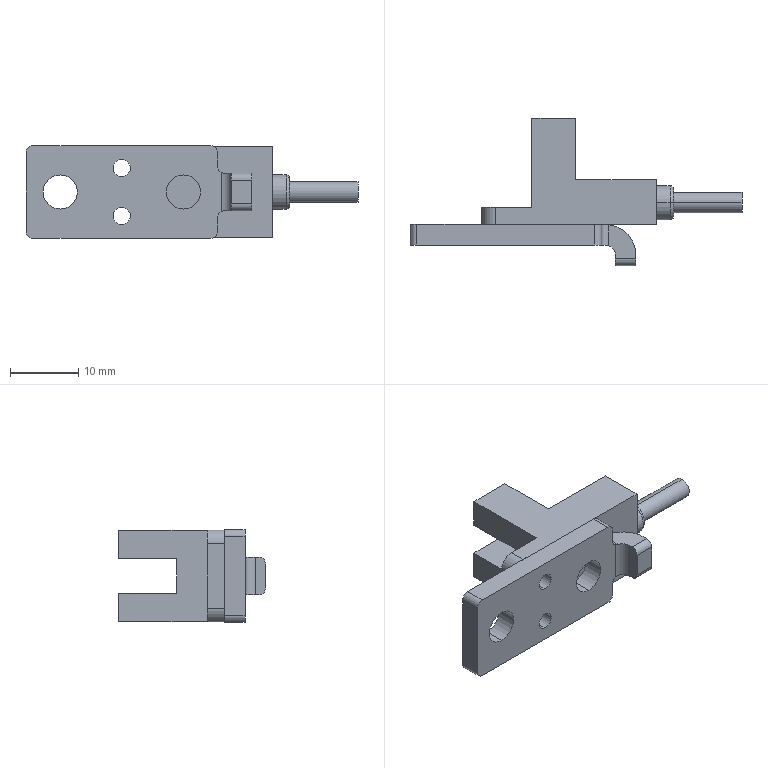Part | STEP file | Copy of 50-sensor^K50A-1H20-S(formula driven)-L1200 right | 2 solids | 58 faces | box 48.5 x 21.5 x 13.5 mm | volume 3491 mm3 | cylinder 28 | plane 28 | spline 2 | commonest cylinder face diameters 2 x8 5 x6 2.5 x4 3.5 x4 3 x3 4 x2